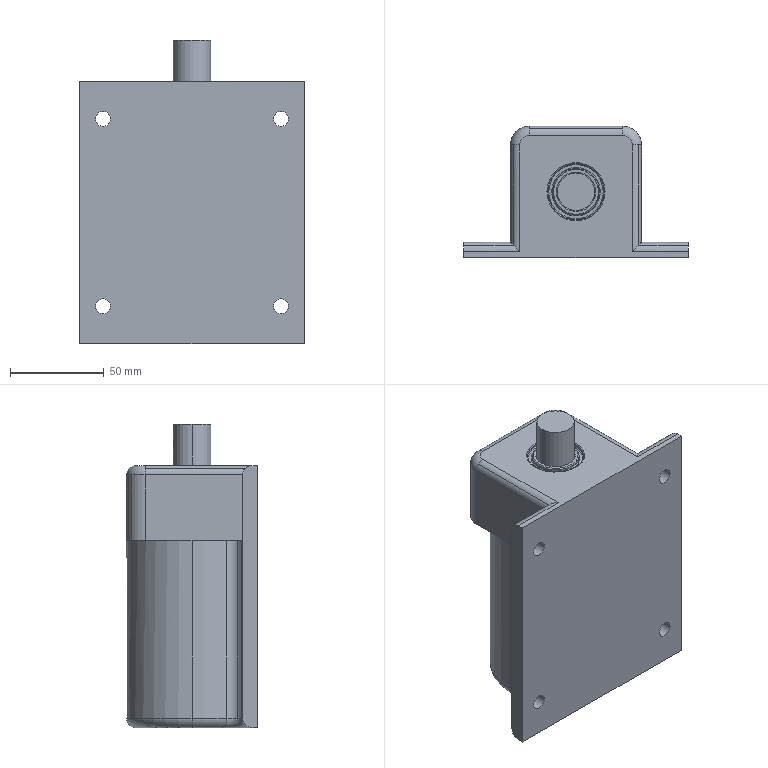Part | SolidWorks | features BaseBody 1 | 1 solid | 78 faces | box 120 x 70 x 162 mm | volume 674674 mm3 | cylinder 43 | plane 19 | torus 16 | commonest cylinder face diameters 10 x14 8 x8 20 x6 11 x4 70 x3 4 x2